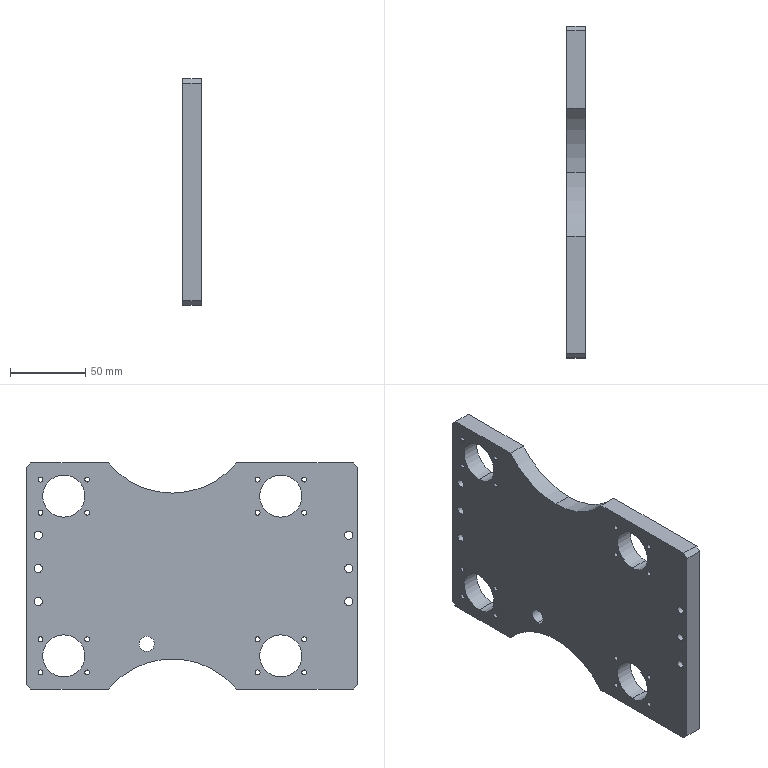Part | STEP file | support plate 26_SUS304 | 1 solid | 87 faces | box 12 x 220 x 150 mm | volume 331927 mm3 | cylinder 69 | plane 18 | commonest cylinder face diameters 3.3 x32 5.5 x12 10 x12 28 x8 110 x3 10.2 x2